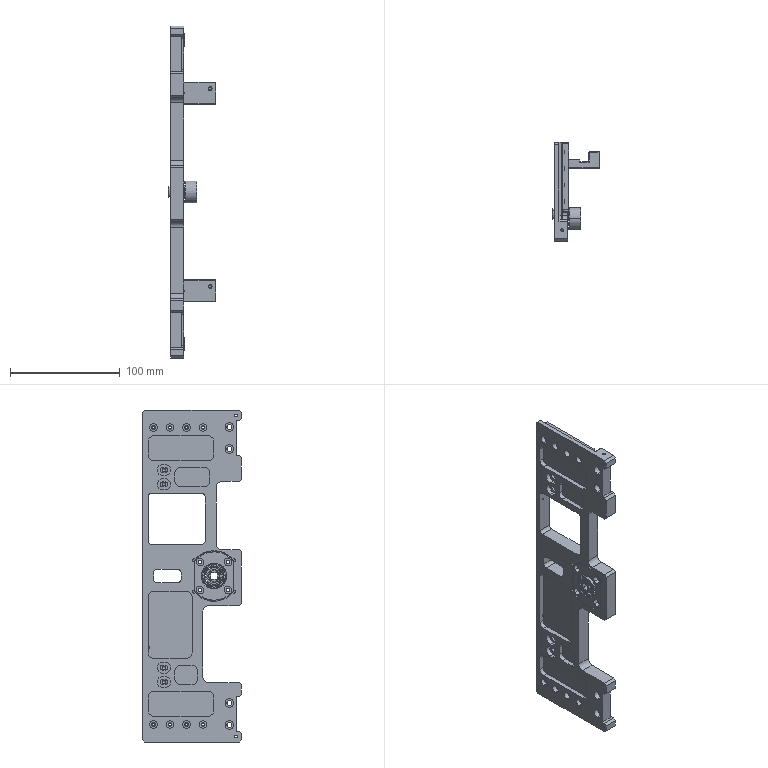Part | NX | features BREP 10 | 14 solids | 894 faces | box 43 x 90 x 302 mm | volume 186780 mm3 | cylinder 375 | plane 375 | cone 56 | sphere 56 | torus 32 | commonest cylinder face diameters 2.5 x60 10 x58 4.4 x32 3.4 x24 7 x24 4.5 x16